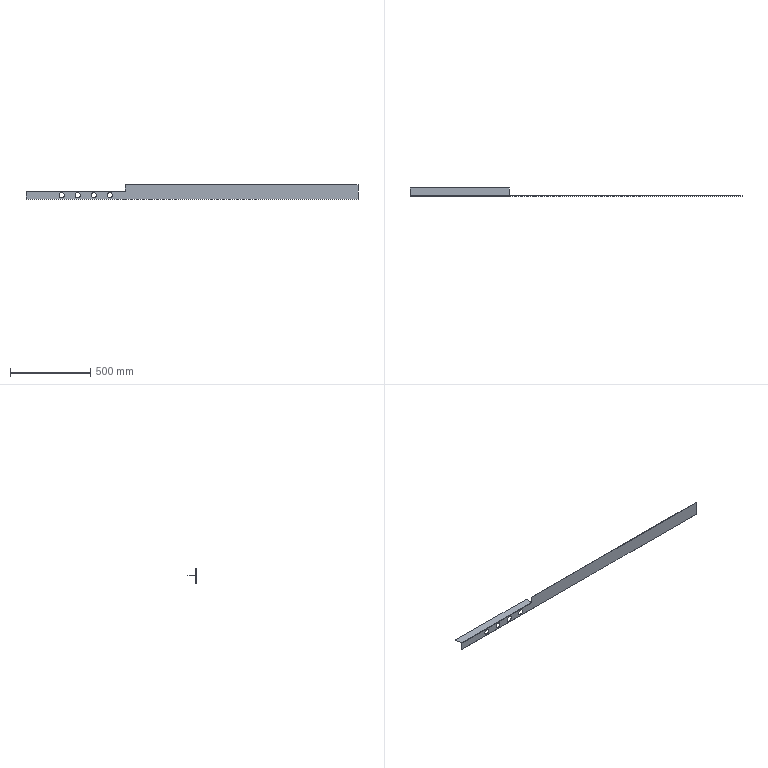Part | STEP file | Baffle 3 | 1 solid | 28 faces | box 2070 x 50 x 90 mm | volume 281521 mm3 | plane 18 | cylinder 10 | commonest cylinder face diameters 33 x8 2 x1 5 x1
STEP:
#1=CARTESIAN_POINT('',(522.5,-1.5,-41.5));
#2=VERTEX_POINT('',#1);
#3=CARTESIAN_POINT('',(522.5,-1.5,-8.5));
#4=VERTEX_POINT('',#3);
#5=CARTESIAN_POINT('',(522.5,-1.5,-25.));
#6=DIRECTION('',(0.,1.,0.));
#7=DIRECTION('',(0.,0.,1.));
#8=AXIS2_PLACEMENT_3D('',#5,#6,#7);
#9=CIRCLE('',#8,16.5);
#10=EDGE_CURVE('',#2,#4,#9,.T.);
#11=ORIENTED_EDGE('',*,*,#10,.F.);
#12=CARTESIAN_POINT('',(522.5,0.,-41.5));
#13=VERTEX_POINT('',#12);
#14=CARTESIAN_POINT('',(522.5,-10.,-41.5));
#15=DIRECTION('',(0.,1.,0.));
#16=VECTOR('',#15,1000.);
#17=LINE('',#14,#16);
#18=EDGE_CURVE('',#2,#13,#17,.T.);
#19=ORIENTED_EDGE('',*,*,#18,.T.);
#20=CARTESIAN_POINT('',(522.5,0.,-8.5));
#21=VERTEX_POINT('',#20);
#22=CARTESIAN_POINT('',(522.5,0.,-25.));
#23=DIRECTION('',(0.,1.,0.));
#24=DIRECTION('',(0.,0.,1.));
#25=AXIS2_PLACEMENT_3D('',#22,#23,#24);
#26=CIRCLE('',#25,16.5);
#27=EDGE_CURVE('',#13,#21,#26,.T.);
#28=ORIENTED_EDGE('',*,*,#27,.T.);
#29=CARTESIAN_POINT('',(522.5,-10.,-8.5));
#30=DIRECTION('',(0.,1.,0.));
#31=VECTOR('',#30,1000.);
#32=LINE('',#29,#31);
#33=EDGE_CURVE('',#4,#21,#32,.T.);
#34=ORIENTED_EDGE('',*,*,#33,.F.);
#35=EDGE_LOOP('',(#11,#19,#28,#34));
#36=FACE_OUTER_BOUND('',#35,.T.);
#37=CARTESIAN_POINT('',(522.5,-10.,-25.));
#38=DIRECTION('',(0.,1.,0.));
#39=DIRECTION('',(0.,0.,1.));
#40=AXIS2_PLACEMENT_3D('',#37,#38,#39);
#41=CYLINDRICAL_SURFACE('',#40,16.5);
#42=ADVANCED_FACE('',(#36),#41,.F.);
#43=CARTESIAN_POINT('',(422.5,-1.5,-41.5));
#44=VERTEX_POINT('',#43);
#45=CARTESIAN_POINT('',(422.5,-1.5,-8.5));
#46=VERTEX_POINT('',#45);
#47=CARTESIAN_POINT('',(422.5,-1.5,-25.));
#48=DIRECTION('',(0.,1.,0.));
#49=DIRECTION('',(0.,0.,1.));
#50=AXIS2_PLACEMENT_3D('',#47,#48,#49);
#51=CIRCLE('',#50,16.5);
#52=EDGE_CURVE('',#44,#46,#51,.T.);
#53=ORIENTED_EDGE('',*,*,#52,.F.);
#54=CARTESIAN_POINT('',(422.5,0.,-41.5));
#55=VERTEX_POINT('',#54);
#56=CARTESIAN_POINT('',(422.5,-10.,-41.5));
#57=DIRECTION('',(0.,1.,0.));
#58=VECTOR('',#57,1000.);
#59=LINE('',#56,#58);
#60=EDGE_CURVE('',#44,#55,#59,.T.);
#61=ORIENTED_EDGE('',*,*,#60,.T.);
#62=CARTESIAN_POINT('',(422.5,0.,-8.5));
#63=VERTEX_POINT('',#62);
#64=CARTESIAN_POINT('',(422.5,0.,-25.));
#65=DIRECTION('',(0.,1.,0.));
#66=DIRECTION('',(0.,0.,1.));
#67=AXIS2_PLACEMENT_3D('',#64,#65,#66);
#68=CIRCLE('',#67,16.5);
#69=EDGE_CURVE('',#55,#63,#68,.T.);
#70=ORIENTED_EDGE('',*,*,#69,.T.);
#71=CARTESIAN_POINT('',(422.5,-10.,-8.5));
#72=DIRECTION('',(0.,1.,0.));
#73=VECTOR('',#72,1000.);
#74=LINE('',#71,#73);
#75=EDGE_CURVE('',#46,#63,#74,.T.);
#76=ORIENTED_EDGE('',*,*,#75,.F.);
#77=EDGE_LOOP('',(#53,#61,#70,#76));
#78=FACE_OUTER_BOUND('',#77,.T.);
#79=CARTESIAN_POINT('',(422.5,-10.,-25.));
#80=DIRECTION('',(0.,1.,0.));
#81=DIRECTION('',(0.,0.,1.));
#82=AXIS2_PLACEMENT_3D('',#79,#80,#81);
#83=CYLINDRICAL_SURFACE('',#82,16.5);
#84=ADVANCED_FACE('',(#78),#83,.F.);
#85=CARTESIAN_POINT('',(322.5,-1.5,-41.5));
#86=VERTEX_POINT('',#85);
#87=CARTESIAN_POINT('',(322.5,-1.5,-8.5));
#88=VERTEX_POINT('',#87);
#89=CARTESIAN_POINT('',(322.5,-1.5,-25.));
#90=DIRECTION('',(0.,1.,0.));
#91=DIRECTION('',(0.,0.,1.));
#92=AXIS2_PLACEMENT_3D('',#89,#90,#91);
#93=CIRCLE('',#92,16.5);
#94=EDGE_CURVE('',#86,#88,#93,.T.);
#95=ORIENTED_EDGE('',*,*,#94,.F.);
#96=CARTESIAN_POINT('',(322.5,0.,-41.5));
#97=VERTEX_POINT('',#96);
#98=CARTESIAN_POINT('',(322.5,-10.,-41.5));
#99=DIRECTION('',(0.,1.,0.));
#100=VECTOR('',#99,1000.);
#101=LINE('',#98,#100);
#102=EDGE_CURVE('',#86,#97,#101,.T.);
#103=ORIENTED_EDGE('',*,*,#102,.T.);
#104=CARTESIAN_POINT('',(322.5,0.,-8.5));
#105=VERTEX_POINT('',#104);
#106=CARTESIAN_POINT('',(322.5,0.,-25.));
#107=DIRECTION('',(0.,1.,0.));
#108=DIRECTION('',(0.,0.,1.));
#109=AXIS2_PLACEMENT_3D('',#106,#107,#108);
#110=CIRCLE('',#109,16.5);
#111=EDGE_CURVE('',#97,#105,#110,.T.);
#112=ORIENTED_EDGE('',*,*,#111,.T.);
#113=CARTESIAN_POINT('',(322.5,-10.,-8.5));
#114=DIRECTION('',(0.,1.,0.));
#115=VECTOR('',#114,1000.);
#116=LINE('',#113,#115);
#117=EDGE_CURVE('',#88,#105,#116,.T.);
#118=ORIENTED_EDGE('',*,*,#117,.F.);
#119=EDGE_LOOP('',(#95,#103,#112,#118));
#120=FACE_OUTER_BOUND('',#119,.T.);
#121=CARTESIAN_POINT('',(322.5,-10.,-25.));
#122=DIRECTION('',(0.,1.,0.));
#123=DIRECTION('',(0.,0.,1.));
#124=AXIS2_PLACEMENT_3D('',#121,#122,#123);
#125=CYLINDRICAL_SURFACE('',#124,16.5);
#126=ADVANCED_FACE('',(#120),#125,.F.);
#127=CARTESIAN_POINT('',(222.5,-1.5,-41.5));
#128=VERTEX_POINT('',#127);
#129=CARTESIAN_POINT('',(222.5,-1.5,-8.5));
#130=VERTEX_POINT('',#129);
#131=CARTESIAN_POINT('',(222.5,-1.5,-25.));
#132=DIRECTION('',(0.,1.,0.));
#133=DIRECTION('',(0.,0.,1.));
#134=AXIS2_PLACEMENT_3D('',#131,#132,#133);
#135=CIRCLE('',#134,16.5);
#136=EDGE_CURVE('',#128,#130,#135,.T.);
#137=ORIENTED_EDGE('',*,*,#136,.F.);
#138=CARTESIAN_POINT('',(222.5,0.,-41.5));
#139=VERTEX_POINT('',#138);
#140=CARTESIAN_POINT('',(222.5,-10.,-41.5));
#141=DIRECTION('',(0.,1.,0.));
#142=VECTOR('',#141,1000.);
#143=LINE('',#140,#142);
#144=EDGE_CURVE('',#128,#139,#143,.T.);
#145=ORIENTED_EDGE('',*,*,#144,.T.);
#146=CARTESIAN_POINT('',(222.5,0.,-8.5));
#147=VERTEX_POINT('',#146);
#148=CARTESIAN_POINT('',(222.5,0.,-25.));
#149=DIRECTION('',(0.,1.,0.));
#150=DIRECTION('',(0.,0.,1.));
#151=AXIS2_PLACEMENT_3D('',#148,#149,#150);
#152=CIRCLE('',#151,16.5);
#153=EDGE_CURVE('',#139,#147,#152,.T.);
#154=ORIENTED_EDGE('',*,*,#153,.T.);
#155=CARTESIAN_POINT('',(222.5,-10.,-8.5));
#156=DIRECTION('',(0.,1.,0.));
#157=VECTOR('',#156,1000.);
#158=LINE('',#155,#157);
#159=EDGE_CURVE('',#130,#147,#158,.T.);
#160=ORIENTED_EDGE('',*,*,#159,.F.);
#161=EDGE_LOOP('',(#137,#145,#154,#160));
#162=FACE_OUTER_BOUND('',#161,.T.);
#163=CARTESIAN_POINT('',(222.5,-10.,-25.));
#164=DIRECTION('',(0.,1.,0.));
#165=DIRECTION('',(0.,0.,1.));
#166=AXIS2_PLACEMENT_3D('',#163,#164,#165);
#167=CYLINDRICAL_SURFACE('',#166,16.5);
#168=ADVANCED_FACE('',(#162),#167,.F.);
#169=CARTESIAN_POINT('',(522.5,-1.5,-25.));
#170=DIRECTION('',(0.,1.,0.));
#171=DIRECTION('',(0.,0.,1.));
#172=AXIS2_PLACEMENT_3D('',#169,#170,#171);
#173=CIRCLE('',#172,16.5);
#174=EDGE_CURVE('',#4,#2,#173,.T.);
#175=ORIENTED_EDGE('',*,*,#174,.T.);
#176=ORIENTED_EDGE('',*,*,#10,.T.);
#177=EDGE_LOOP('',(#175,#176));
#178=FACE_BOUND('',#177,.T.);
#179=CARTESIAN_POINT('',(422.5,-1.5,-25.));
#180=DIRECTION('',(0.,1.,0.));
#181=DIRECTION('',(0.,0.,1.));
#182=AXIS2_PLACEMENT_3D('',#179,#180,#181);
#183=CIRCLE('',#182,16.5);
#184=EDGE_CURVE('',#46,#44,#183,.T.);
#185=ORIENTED_EDGE('',*,*,#184,.T.);
#186=ORIENTED_EDGE('',*,*,#52,.T.);
#187=EDGE_LOOP('',(#185,#186));
#188=FACE_BOUND('',#187,.T.);
#189=CARTESIAN_POINT('',(322.5,-1.5,-25.));
#190=DIRECTION('',(0.,1.,0.));
#191=DIRECTION('',(0.,0.,1.));
#192=AXIS2_PLACEMENT_3D('',#189,#190,#191);
#193=CIRCLE('',#192,16.5);
#194=EDGE_CURVE('',#88,#86,#193,.T.);
#195=ORIENTED_EDGE('',*,*,#194,.T.);
#196=ORIENTED_EDGE('',*,*,#94,.T.);
#197=EDGE_LOOP('',(#195,#196));
#198=FACE_BOUND('',#197,.T.);
#199=CARTESIAN_POINT('',(222.5,-1.5,-25.));
#200=DIRECTION('',(0.,1.,0.));
#201=DIRECTION('',(0.,0.,1.));
#202=AXIS2_PLACEMENT_3D('',#199,#200,#201);
#203=CIRCLE('',#202,16.5);
#204=EDGE_CURVE('',#130,#128,#203,.T.);
#205=ORIENTED_EDGE('',*,*,#204,.T.);
#206=ORIENTED_EDGE('',*,*,#136,.T.);
#207=EDGE_LOOP('',(#205,#206));
#208=FACE_BOUND('',#207,.T.);
#209=CARTESIAN_POINT('',(620.75,-1.5,0.));
#210=VERTEX_POINT('',#209);
#211=CARTESIAN_POINT('',(620.,-1.5,0.));
#212=VERTEX_POINT('',#211);
#213=CARTESIAN_POINT('',(0.,-1.5,0.));
#214=DIRECTION('',(-1.,0.,0.));
#215=VECTOR('',#214,1000.);
#216=LINE('',#213,#215);
#217=EDGE_CURVE('',#210,#212,#216,.T.);
#218=ORIENTED_EDGE('',*,*,#217,.F.);
#219=CARTESIAN_POINT('',(620.75,-1.5,-3.25));
#220=VERTEX_POINT('',#219);
#221=CARTESIAN_POINT('',(620.75,-1.5,0.));
#222=DIRECTION('',(0.,0.,1.));
#223=VECTOR('',#222,1000.);
#224=LINE('',#221,#223);
#225=EDGE_CURVE('',#220,#210,#224,.T.);
#226=ORIENTED_EDGE('',*,*,#225,.F.);
#227=CARTESIAN_POINT('',(620.,-1.5,-3.25));
#228=VERTEX_POINT('',#227);
#229=CARTESIAN_POINT('',(0.,-1.5,-3.25));
#230=DIRECTION('',(1.,0.,0.));
#231=VECTOR('',#230,1000.);
#232=LINE('',#229,#231);
#233=EDGE_CURVE('',#228,#220,#232,.T.);
#234=ORIENTED_EDGE('',*,*,#233,.F.);
#235=CARTESIAN_POINT('',(620.,-1.5,-2.5));
#236=VERTEX_POINT('',#235);
#237=CARTESIAN_POINT('',(620.,-1.5,0.));
#238=DIRECTION('',(0.,0.,-1.));
#239=VECTOR('',#238,1000.);
#240=LINE('',#237,#239);
#241=EDGE_CURVE('',#236,#228,#240,.T.);
#242=ORIENTED_EDGE('',*,*,#241,.F.);
#243=CARTESIAN_POINT('',(0.,-1.5,-2.5));
#244=VERTEX_POINT('',#243);
#245=CARTESIAN_POINT('',(620.,-1.5,-2.5));
#246=DIRECTION('',(-1.,0.,0.));
#247=VECTOR('',#246,1000.);
#248=LINE('',#245,#247);
#249=EDGE_CURVE('',#236,#244,#248,.T.);
#250=ORIENTED_EDGE('',*,*,#249,.T.);
#251=CARTESIAN_POINT('',(0.,-1.5,-50.));
#252=VERTEX_POINT('',#251);
#253=CARTESIAN_POINT('',(0.,-1.5,-50.));
#254=DIRECTION('',(0.,0.,1.));
#255=VECTOR('',#254,1000.);
#256=LINE('',#253,#255);
#257=EDGE_CURVE('',#252,#244,#256,.T.);
#258=ORIENTED_EDGE('',*,*,#257,.F.);
#259=CARTESIAN_POINT('',(2070.,-1.5,-50.));
#260=VERTEX_POINT('',#259);
#261=CARTESIAN_POINT('',(2070.,-1.5,-50.));
#262=DIRECTION('',(-1.,0.,0.));
#263=VECTOR('',#262,1000.);
#264=LINE('',#261,#263);
#265=EDGE_CURVE('',#260,#252,#264,.T.);
#266=ORIENTED_EDGE('',*,*,#265,.F.);
#267=CARTESIAN_POINT('',(2070.,-1.5,40.));
#268=VERTEX_POINT('',#267);
#269=CARTESIAN_POINT('',(2070.,-1.5,40.));
#270=DIRECTION('',(0.,0.,-1.));
#271=VECTOR('',#270,1000.);
#272=LINE('',#269,#271);
#273=EDGE_CURVE('',#268,#260,#272,.T.);
#274=ORIENTED_EDGE('',*,*,#273,.F.);
#275=CARTESIAN_POINT('',(620.,-1.5,40.));
#276=VERTEX_POINT('',#275);
#277=CARTESIAN_POINT('',(620.,-1.5,40.));
#278=DIRECTION('',(1.,0.,0.));
#279=VECTOR('',#278,1000.);
#280=LINE('',#277,#279);
#281=EDGE_CURVE('',#276,#268,#280,.T.);
#282=ORIENTED_EDGE('',*,*,#281,.F.);
#283=CARTESIAN_POINT('',(620.,-1.5,0.));
#284=DIRECTION('',(0.,0.,1.));
#285=VECTOR('',#284,1000.);
#286=LINE('',#283,#285);
#287=EDGE_CURVE('',#212,#276,#286,.T.);
#288=ORIENTED_EDGE('',*,*,#287,.F.);
#289=EDGE_LOOP('',(#218,#226,#234,#242,#250,#258,#266,#274,#282,#288));
#290=FACE_OUTER_BOUND('',#289,.T.);
#291=CARTESIAN_POINT('',(0.,-1.5,0.));
#292=DIRECTION('',(0.,1.,0.));
#293=DIRECTION('',(0.,0.,1.));
#294=AXIS2_PLACEMENT_3D('',#291,#292,#293);
#295=PLANE('',#294);
#296=ADVANCED_FACE('',(#178,#188,#198,#208,#290),#295,.F.);
#297=CARTESIAN_POINT('',(522.5,0.,-25.));
#298=DIRECTION('',(0.,1.,0.));
#299=DIRECTION('',(0.,0.,1.));
#300=AXIS2_PLACEMENT_3D('',#297,#298,#299);
#301=CIRCLE('',#300,16.5);
#302=EDGE_CURVE('',#21,#13,#301,.T.);
#303=ORIENTED_EDGE('',*,*,#302,.F.);
#304=ORIENTED_EDGE('',*,*,#27,.F.);
#305=EDGE_LOOP('',(#303,#304));
#306=FACE_BOUND('',#305,.T.);
#307=CARTESIAN_POINT('',(422.5,0.,-25.));
#308=DIRECTION('',(0.,1.,0.));
#309=DIRECTION('',(0.,0.,1.));
#310=AXIS2_PLACEMENT_3D('',#307,#308,#309);
#311=CIRCLE('',#310,16.5);
#312=EDGE_CURVE('',#63,#55,#311,.T.);
#313=ORIENTED_EDGE('',*,*,#312,.F.);
#314=ORIENTED_EDGE('',*,*,#69,.F.);
#315=EDGE_LOOP('',(#313,#314));
#316=FACE_BOUND('',#315,.T.);
#317=CARTESIAN_POINT('',(322.5,0.,-25.));
#318=DIRECTION('',(0.,1.,0.));
#319=DIRECTION('',(0.,0.,1.));
#320=AXIS2_PLACEMENT_3D('',#317,#318,#319);
#321=CIRCLE('',#320,16.5);
#322=EDGE_CURVE('',#105,#97,#321,.T.);
#323=ORIENTED_EDGE('',*,*,#322,.F.);
#324=ORIENTED_EDGE('',*,*,#111,.F.);
#325=EDGE_LOOP('',(#323,#324));
#326=FACE_BOUND('',#325,.T.);
#327=CARTESIAN_POINT('',(222.5,0.,-25.));
#328=DIRECTION('',(0.,1.,0.));
#329=DIRECTION('',(0.,0.,1.));
#330=AXIS2_PLACEMENT_3D('',#327,#328,#329);
#331=CIRCLE('',#330,16.5);
#332=EDGE_CURVE('',#147,#139,#331,.T.);
#333=ORIENTED_EDGE('',*,*,#332,.F.);
#334=ORIENTED_EDGE('',*,*,#153,.F.);
#335=EDGE_LOOP('',(#333,#334));
#336=FACE_BOUND('',#335,.T.);
#337=CARTESIAN_POINT('',(620.75,0.,0.));
#338=VERTEX_POINT('',#337);
#339=CARTESIAN_POINT('',(620.75,0.,-3.25));
#340=VERTEX_POINT('',#339);
#341=CARTESIAN_POINT('',(620.75,0.,0.));
#342=DIRECTION('',(0.,0.,-1.));
#343=VECTOR('',#342,1000.);
#344=LINE('',#341,#343);
#345=EDGE_CURVE('',#338,#340,#344,.T.);
#346=ORIENTED_EDGE('',*,*,#345,.F.);
#347=CARTESIAN_POINT('',(620.,0.,0.));
#348=VERTEX_POINT('',#347);
#349=CARTESIAN_POINT('',(620.,0.,0.));
#350=DIRECTION('',(1.,0.,0.));
#351=VECTOR('',#350,1000.);
#352=LINE('',#349,#351);
#353=EDGE_CURVE('',#348,#338,#352,.T.);
#354=ORIENTED_EDGE('',*,*,#353,.F.);
#355=CARTESIAN_POINT('',(620.,0.,40.));
#356=VERTEX_POINT('',#355);
#357=CARTESIAN_POINT('',(620.,0.,0.));
#358=DIRECTION('',(0.,0.,1.));
#359=VECTOR('',#358,1000.);
#360=LINE('',#357,#359);
#361=EDGE_CURVE('',#348,#356,#360,.T.);
#362=ORIENTED_EDGE('',*,*,#361,.T.);
#363=CARTESIAN_POINT('',(2070.,0.,40.));
#364=VERTEX_POINT('',#363);
#365=CARTESIAN_POINT('',(620.,0.,40.));
#366=DIRECTION('',(1.,0.,0.));
#367=VECTOR('',#366,1000.);
#368=LINE('',#365,#367);
#369=EDGE_CURVE('',#356,#364,#368,.T.);
#370=ORIENTED_EDGE('',*,*,#369,.T.);
#371=CARTESIAN_POINT('',(2070.,0.,-50.));
#372=VERTEX_POINT('',#371);
#373=CARTESIAN_POINT('',(2070.,0.,40.));
#374=DIRECTION('',(0.,0.,-1.));
#375=VECTOR('',#374,1000.);
#376=LINE('',#373,#375);
#377=EDGE_CURVE('',#364,#372,#376,.T.);
#378=ORIENTED_EDGE('',*,*,#377,.T.);
#379=CARTESIAN_POINT('',(0.,0.,-50.));
#380=VERTEX_POINT('',#379);
#381=CARTESIAN_POINT('',(2070.,0.,-50.));
#382=DIRECTION('',(-1.,0.,0.));
#383=VECTOR('',#382,1000.);
#384=LINE('',#381,#383);
#385=EDGE_CURVE('',#372,#380,#384,.T.);
#386=ORIENTED_EDGE('',*,*,#385,.T.);
#387=CARTESIAN_POINT('',(0.,0.,-2.5));
#388=VERTEX_POINT('',#387);
#389=CARTESIAN_POINT('',(0.,0.,-50.));
#390=DIRECTION('',(0.,0.,1.));
#391=VECTOR('',#390,1000.);
#392=LINE('',#389,#391);
#393=EDGE_CURVE('',#380,#388,#392,.T.);
#394=ORIENTED_EDGE('',*,*,#393,.T.);
#395=CARTESIAN_POINT('',(620.,0.,-2.5));
#396=VERTEX_POINT('',#395);
#397=CARTESIAN_POINT('',(620.,0.,-2.5));
#398=DIRECTION('',(-1.,0.,0.));
#399=VECTOR('',#398,1000.);
#400=LINE('',#397,#399);
#401=EDGE_CURVE('',#396,#388,#400,.T.);
#402=ORIENTED_EDGE('',*,*,#401,.F.);
#403=CARTESIAN_POINT('',(620.,0.,-3.25));
#404=VERTEX_POINT('',#403);
#405=CARTESIAN_POINT('',(620.,0.,-3.25));
#406=DIRECTION('',(0.,0.,1.));
#407=VECTOR('',#406,1000.);
#408=LINE('',#405,#407);
#409=EDGE_CURVE('',#404,#396,#408,.T.);
#410=ORIENTED_EDGE('',*,*,#409,.F.);
#411=CARTESIAN_POINT('',(620.75,0.,-3.25));
#412=DIRECTION('',(-1.,0.,0.));
#413=VECTOR('',#412,1000.);
#414=LINE('',#411,#413);
#415=EDGE_CURVE('',#340,#404,#414,.T.);
#416=ORIENTED_EDGE('',*,*,#415,.F.);
#417=EDGE_LOOP('',(#346,#354,#362,#370,#378,#386,#394,#402,#410,#416));
#418=FACE_OUTER_BOUND('',#417,.T.);
#419=CARTESIAN_POINT('',(0.,0.,0.));
#420=DIRECTION('',(0.,1.,0.));
#421=DIRECTION('',(0.,0.,1.));
#422=AXIS2_PLACEMENT_3D('',#419,#420,#421);
#423=PLANE('',#422);
#424=ADVANCED_FACE('',(#306,#316,#326,#336,#418),#423,.T.);
#425=CARTESIAN_POINT('',(0.,0.,-2.5));
#426=DIRECTION('',(0.,-1.,0.));
#427=VECTOR('',#426,1000.);
#428=LINE('',#425,#427);
#429=EDGE_CURVE('',#388,#244,#428,.T.);
#430=ORIENTED_EDGE('',*,*,#429,.F.);
#431=ORIENTED_EDGE('',*,*,#393,.F.);
#432=CARTESIAN_POINT('',(0.,-1.5,-50.));
#433=DIRECTION('',(0.,1.,0.));
#434=VECTOR('',#433,1000.);
#435=LINE('',#432,#434);
#436=EDGE_CURVE('',#252,#380,#435,.T.);
#437=ORIENTED_EDGE('',*,*,#436,.F.);
#438=ORIENTED_EDGE('',*,*,#257,.T.);
#439=EDGE_LOOP('',(#430,#431,#437,#438));
#440=FACE_OUTER_BOUND('',#439,.T.);
#441=CARTESIAN_POINT('',(0.,-1.5,-50.));
#442=DIRECTION('',(-1.,0.,0.));
#443=DIRECTION('',(0.,0.,1.));
#444=AXIS2_PLACEMENT_3D('',#441,#442,#443);
#445=PLANE('',#444);
#446=ADVANCED_FACE('',(#440),#445,.T.);
#447=ORIENTED_EDGE('',*,*,#385,.F.);
#448=CARTESIAN_POINT('',(2070.,-1.5,-50.));
#449=DIRECTION('',(0.,1.,0.));
#450=VECTOR('',#449,1000.);
#451=LINE('',#448,#450);
#452=EDGE_CURVE('',#260,#372,#451,.T.);
#453=ORIENTED_EDGE('',*,*,#452,.F.);
#454=ORIENTED_EDGE('',*,*,#265,.T.);
#455=ORIENTED_EDGE('',*,*,#436,.T.);
#456=EDGE_LOOP('',(#447,#453,#454,#455));
#457=FACE_OUTER_BOUND('',#456,.T.);
#458=CARTESIAN_POINT('',(2070.,-1.5,-50.));
#459=DIRECTION('',(0.,0.,-1.));
#460=DIRECTION('',(-1.,0.,0.));
#461=AXIS2_PLACEMENT_3D('',#458,#459,#460);
#462=PLANE('',#461);
#463=ADVANCED_FACE('',(#457),#462,.T.);
#464=ORIENTED_EDGE('',*,*,#377,.F.);
#465=CARTESIAN_POINT('',(2070.,-1.5,40.));
#466=DIRECTION('',(0.,1.,0.));
#467=VECTOR('',#466,1000.);
#468=LINE('',#465,#467);
#469=EDGE_CURVE('',#268,#364,#468,.T.);
#470=ORIENTED_EDGE('',*,*,#469,.F.);
#471=ORIENTED_EDGE('',*,*,#273,.T.);
#472=ORIENTED_EDGE('',*,*,#452,.T.);
#473=EDGE_LOOP('',(#464,#470,#471,#472));
#474=FACE_OUTER_BOUND('',#473,.T.);
#475=CARTESIAN_POINT('',(2070.,-1.5,40.));
#476=DIRECTION('',(1.,0.,0.));
#477=DIRECTION('',(0.,0.,-1.));
#478=AXIS2_PLACEMENT_3D('',#475,#476,#477);
#479=PLANE('',#478);
#480=ADVANCED_FACE('',(#474),#479,.T.);
#481=ORIENTED_EDGE('',*,*,#369,.F.);
#482=CARTESIAN_POINT('',(620.,-1.5,40.));
#483=DIRECTION('',(0.,1.,0.));
#484=VECTOR('',#483,1000.);
#485=LINE('',#482,#484);
#486=EDGE_CURVE('',#276,#356,#485,.T.);
#487=ORIENTED_EDGE('',*,*,#486,.F.);
#488=ORIENTED_EDGE('',*,*,#281,.T.);
#489=ORIENTED_EDGE('',*,*,#469,.T.);
#490=EDGE_LOOP('',(#481,#487,#488,#489));
#491=FACE_OUTER_BOUND('',#490,.T.);
#492=CARTESIAN_POINT('',(620.,-1.5,40.));
#493=DIRECTION('',(0.,0.,1.));
#494=DIRECTION('',(1.,0.,0.));
#495=AXIS2_PLACEMENT_3D('',#492,#493,#494);
#496=PLANE('',#495);
#497=ADVANCED_FACE('',(#491),#496,.T.);
#498=ORIENTED_EDGE('',*,*,#361,.F.);
#499=CARTESIAN_POINT('',(620.,-1.5,0.));
#500=DIRECTION('',(0.,1.,0.));
#501=VECTOR('',#500,1000.);
#502=LINE('',#499,#501);
#503=EDGE_CURVE('',#212,#348,#502,.T.);
#504=ORIENTED_EDGE('',*,*,#503,.F.);
#505=ORIENTED_EDGE('',*,*,#287,.T.);
#506=ORIENTED_EDGE('',*,*,#486,.T.);
#507=EDGE_LOOP('',(#498,#504,#505,#506));
#508=FACE_OUTER_BOUND('',#507,.T.);
#509=CARTESIAN_POINT('',(620.,-1.5,0.));
#510=DIRECTION('',(-1.,0.,0.));
#511=DIRECTION('',(0.,0.,1.));
#512=AXIS2_PLACEMENT_3D('',#509,#510,#511);
#513=PLANE('',#512);
#514=ADVANCED_FACE('',(#508),#513,.T.);
#515=CARTESIAN_POINT('',(620.75,0.,0.));
#516=DIRECTION('',(0.,-1.,0.));
#517=VECTOR('',#516,1000.);
#518=LINE('',#515,#517);
#519=EDGE_CURVE('',#338,#210,#518,.T.);
#520=ORIENTED_EDGE('',*,*,#519,.T.);
#521=ORIENTED_EDGE('',*,*,#217,.T.);
#522=ORIENTED_EDGE('',*,*,#503,.T.);
#523=ORIENTED_EDGE('',*,*,#353,.T.);
#524=EDGE_LOOP('',(#520,#521,#522,#523));
#525=FACE_OUTER_BOUND('',#524,.T.);
#526=CARTESIAN_POINT('',(620.,0.,0.));
#527=DIRECTION('',(0.,0.,-1.));
#528=DIRECTION('',(0.,1.,0.));
#529=AXIS2_PLACEMENT_3D('',#526,#527,#528);
#530=PLANE('',#529);
#531=ADVANCED_FACE('',(#525),#530,.T.);
#532=CARTESIAN_POINT('',(620.75,0.,-3.25));
#533=DIRECTION('',(0.,-1.,0.));
#534=VECTOR('',#533,1000.);
#535=LINE('',#532,#534);
#536=EDGE_CURVE('',#340,#220,#535,.T.);
#537=ORIENTED_EDGE('',*,*,#536,.T.);
#538=ORIENTED_EDGE('',*,*,#225,.T.);
#539=ORIENTED_EDGE('',*,*,#519,.F.);
#540=ORIENTED_EDGE('',*,*,#345,.T.);
#541=EDGE_LOOP('',(#537,#538,#539,#540));
#542=FACE_OUTER_BOUND('',#541,.T.);
#543=CARTESIAN_POINT('',(620.75,0.,0.));
#544=DIRECTION('',(-1.,0.,0.));
#545=DIRECTION('',(0.,0.,1.));
#546=AXIS2_PLACEMENT_3D('',#543,#544,#545);
#547=PLANE('',#546);
#548=ADVANCED_FACE('',(#542),#547,.T.);
#549=CARTESIAN_POINT('',(620.,0.,-3.25));
#550=DIRECTION('',(0.,-1.,0.));
#551=VECTOR('',#550,1000.);
#552=LINE('',#549,#551);
#553=EDGE_CURVE('',#404,#228,#552,.T.);
#554=ORIENTED_EDGE('',*,*,#553,.T.);
#555=ORIENTED_EDGE('',*,*,#233,.T.);
#556=ORIENTED_EDGE('',*,*,#536,.F.);
#557=ORIENTED_EDGE('',*,*,#415,.T.);
#558=EDGE_LOOP('',(#554,#555,#556,#557));
#559=FACE_OUTER_BOUND('',#558,.T.);
#560=CARTESIAN_POINT('',(620.75,0.,-3.25));
#561=DIRECTION('',(0.,0.,1.));
#562=DIRECTION('',(0.,-1.,0.));
#563=AXIS2_PLACEMENT_3D('',#560,#561,#562);
#564=PLANE('',#563);
#565=ADVANCED_FACE('',(#559),#564,.T.);
#566=CARTESIAN_POINT('',(620.,0.,-2.5));
#567=DIRECTION('',(0.,-1.,0.));
#568=VECTOR('',#567,1000.);
#569=LINE('',#566,#568);
#570=EDGE_CURVE('',#396,#236,#569,.T.);
#571=ORIENTED_EDGE('',*,*,#570,.T.);
#572=ORIENTED_EDGE('',*,*,#241,.T.);
#573=ORIENTED_EDGE('',*,*,#553,.F.);
#574=ORIENTED_EDGE('',*,*,#409,.T.);
#575=EDGE_LOOP('',(#571,#572,#573,#574));
#576=FACE_OUTER_BOUND('',#575,.T.);
#577=CARTESIAN_POINT('',(620.,0.,-3.25));
#578=DIRECTION('',(1.,0.,0.));
#579=DIRECTION('',(0.,0.,-1.));
#580=AXIS2_PLACEMENT_3D('',#577,#578,#579);
#581=PLANE('',#580);
#582=ADVANCED_FACE('',(#576),#581,.T.);
#583=CARTESIAN_POINT('',(0.,1.,-1.5));
#584=VERTEX_POINT('',#583);
#585=CARTESIAN_POINT('',(0.,1.,0.));
#586=VERTEX_POINT('',#585);
#587=CARTESIAN_POINT('',(0.,1.,0.));
#588=DIRECTION('',(0.,0.,1.));
#589=VECTOR('',#588,1000.);
#590=LINE('',#587,#589);
#591=EDGE_CURVE('',#584,#586,#590,.T.);
#592=ORIENTED_EDGE('',*,*,#591,.F.);
#593=CARTESIAN_POINT('',(0.,1.,-2.5));
#594=DIRECTION('',(-1.,0.,0.));
#595=DIRECTION('',(0.,0.,-1.));
#596=AXIS2_PLACEMENT_3D('',#593,#594,#595);
#597=CIRCLE('',#596,1.);
#598=EDGE_CURVE('',#388,#584,#597,.T.);
#599=ORIENTED_EDGE('',*,*,#598,.F.);
#600=ORIENTED_EDGE('',*,*,#429,.T.);
#601=CARTESIAN_POINT('',(0.,1.,-2.5));
#602=DIRECTION('',(-1.,0.,0.));
#603=DIRECTION('',(0.,0.,-1.));
#604=AXIS2_PLACEMENT_3D('',#601,#602,#603);
#605=CIRCLE('',#604,2.5);
#606=EDGE_CURVE('',#244,#586,#605,.T.);
#607=ORIENTED_EDGE('',*,*,#606,.T.);
#608=EDGE_LOOP('',(#592,#599,#600,#607));
#609=FACE_OUTER_BOUND('',#608,.T.);
#610=CARTESIAN_POINT('',(0.,1.,-2.5));
#611=DIRECTION('',(-1.,0.,0.));
#612=DIRECTION('',(0.,0.,1.));
#613=AXIS2_PLACEMENT_3D('',#610,#611,#612);
#614=PLANE('',#613);
#615=ADVANCED_FACE('',(#609),#614,.T.);
#616=CARTESIAN_POINT('',(620.,1.,-1.5));
#617=VERTEX_POINT('',#616);
#618=CARTESIAN_POINT('',(620.,1.,-2.5));
#619=DIRECTION('',(1.,0.,0.));
#620=DIRECTION('',(0.,0.,-1.));
#621=AXIS2_PLACEMENT_3D('',#618,#619,#620);
#622=CIRCLE('',#621,1.);
#623=EDGE_CURVE('',#617,#396,#622,.T.);
#624=ORIENTED_EDGE('',*,*,#623,.F.);
#625=CARTESIAN_POINT('',(620.,1.,0.));
#626=VERTEX_POINT('',#625);
#627=CARTESIAN_POINT('',(620.,1.,-1.5));
#628=DIRECTION('',(0.,0.,1.));
#629=VECTOR('',#628,1000.);
#630=LINE('',#627,#629);
#631=EDGE_CURVE('',#617,#626,#630,.T.);
#632=ORIENTED_EDGE('',*,*,#631,.T.);
#633=CARTESIAN_POINT('',(620.,1.,-2.5));
#634=DIRECTION('',(1.,0.,0.));
#635=DIRECTION('',(0.,0.,-1.));
#636=AXIS2_PLACEMENT_3D('',#633,#634,#635);
#637=CIRCLE('',#636,2.5);
#638=EDGE_CURVE('',#626,#236,#637,.T.);
#639=ORIENTED_EDGE('',*,*,#638,.T.);
#640=ORIENTED_EDGE('',*,*,#570,.F.);
#641=EDGE_LOOP('',(#624,#632,#639,#640));
#642=FACE_OUTER_BOUND('',#641,.T.);
#643=CARTESIAN_POINT('',(620.,1.,-2.5));
#644=DIRECTION('',(-1.,0.,0.));
#645=DIRECTION('',(0.,0.,1.));
#646=AXIS2_PLACEMENT_3D('',#643,#644,#645);
#647=PLANE('',#646);
#648=ADVANCED_FACE('',(#642),#647,.F.);
#649=ORIENTED_EDGE('',*,*,#249,.F.);
#650=ORIENTED_EDGE('',*,*,#638,.F.);
#651=CARTESIAN_POINT('',(0.,1.,0.));
#652=DIRECTION('',(-1.,0.,0.));
#653=VECTOR('',#652,1000.);
#654=LINE('',#651,#653);
#655=EDGE_CURVE('',#626,#586,#654,.T.);
#656=ORIENTED_EDGE('',*,*,#655,.T.);
#657=ORIENTED_EDGE('',*,*,#606,.F.);
#658=EDGE_LOOP('',(#649,#650,#656,#657));
#659=FACE_OUTER_BOUND('',#658,.T.);
#660=CARTESIAN_POINT('',(620.,1.,-2.5));
#661=DIRECTION('',(1.,0.,0.));
#662=DIRECTION('',(0.,0.,1.));
#663=AXIS2_PLACEMENT_3D('',#660,#661,#662);
#664=CYLINDRICAL_SURFACE('',#663,2.5);
#665=ADVANCED_FACE('',(#659),#664,.T.);
#666=ORIENTED_EDGE('',*,*,#401,.T.);
#667=ORIENTED_EDGE('',*,*,#598,.T.);
#668=CARTESIAN_POINT('',(0.,1.,-1.5));
#669=DIRECTION('',(1.,0.,0.));
#670=VECTOR('',#669,1000.);
#671=LINE('',#668,#670);
#672=EDGE_CURVE('',#584,#617,#671,.T.);
#673=ORIENTED_EDGE('',*,*,#672,.T.);
#674=ORIENTED_EDGE('',*,*,#623,.T.);
#675=EDGE_LOOP('',(#666,#667,#673,#674));
#676=FACE_OUTER_BOUND('',#675,.T.);
#677=CARTESIAN_POINT('',(620.,1.,-2.5));
#678=DIRECTION('',(1.,0.,0.));
#679=DIRECTION('',(0.,0.,1.));
#680=AXIS2_PLACEMENT_3D('',#677,#678,#679);
#681=CYLINDRICAL_SURFACE('',#680,1.);
#682=ADVANCED_FACE('',(#676),#681,.F.);
#683=ORIENTED_EDGE('',*,*,#591,.T.);
#684=CARTESIAN_POINT('',(0.,48.5,0.));
#685=VERTEX_POINT('',#684);
#686=CARTESIAN_POINT('',(0.,0.,0.));
#687=DIRECTION('',(0.,-1.,0.));
#688=VECTOR('',#687,1000.);
#689=LINE('',#686,#688);
#690=EDGE_CURVE('',#685,#586,#689,.T.);
#691=ORIENTED_EDGE('',*,*,#690,.F.);
#692=CARTESIAN_POINT('',(0.,48.5,-1.5));
#693=VERTEX_POINT('',#692);
#694=CARTESIAN_POINT('',(0.,48.5,0.));
#695=DIRECTION('',(0.,0.,-1.));
#696=VECTOR('',#695,1000.);
#697=LINE('',#694,#696);
#698=EDGE_CURVE('',#685,#693,#697,.T.);
#699=ORIENTED_EDGE('',*,*,#698,.T.);
#700=CARTESIAN_POINT('',(0.,0.,-1.5));
#701=DIRECTION('',(0.,-1.,0.));
#702=VECTOR('',#701,1000.);
#703=LINE('',#700,#702);
#704=EDGE_CURVE('',#693,#584,#703,.T.);
#705=ORIENTED_EDGE('',*,*,#704,.T.);
#706=EDGE_LOOP('',(#683,#691,#699,#705));
#707=FACE_OUTER_BOUND('',#706,.T.);
#708=CARTESIAN_POINT('',(0.,0.,0.));
#709=DIRECTION('',(1.,0.,0.));
#710=DIRECTION('',(0.,0.,-1.));
#711=AXIS2_PLACEMENT_3D('',#708,#709,#710);
#712=PLANE('',#711);
#713=ADVANCED_FACE('',(#707),#712,.F.);
#714=ORIENTED_EDGE('',*,*,#631,.F.);
#715=CARTESIAN_POINT('',(620.,48.5,-1.5));
#716=VERTEX_POINT('',#715);
#717=CARTESIAN_POINT('',(620.,48.5,-1.5));
#718=DIRECTION('',(0.,1.,0.));
#719=VECTOR('',#718,1000.);
#720=LINE('',#717,#719);
#721=EDGE_CURVE('',#617,#716,#720,.T.);
#722=ORIENTED_EDGE('',*,*,#721,.T.);
#723=CARTESIAN_POINT('',(620.,48.5,0.));
#724=VERTEX_POINT('',#723);
#725=CARTESIAN_POINT('',(620.,48.5,0.));
#726=DIRECTION('',(0.,0.,-1.));
#727=VECTOR('',#726,1000.);
#728=LINE('',#725,#727);
#729=EDGE_CURVE('',#724,#716,#728,.T.);
#730=ORIENTED_EDGE('',*,*,#729,.F.);
#731=CARTESIAN_POINT('',(620.,0.,0.));
#732=DIRECTION('',(0.,1.,0.));
#733=VECTOR('',#732,1000.);
#734=LINE('',#731,#733);
#735=EDGE_CURVE('',#626,#724,#734,.T.);
#736=ORIENTED_EDGE('',*,*,#735,.F.);
#737=EDGE_LOOP('',(#714,#722,#730,#736));
#738=FACE_OUTER_BOUND('',#737,.T.);
#739=CARTESIAN_POINT('',(620.,48.5,0.));
#740=DIRECTION('',(-1.,0.,0.));
#741=DIRECTION('',(0.,0.,1.));
#742=AXIS2_PLACEMENT_3D('',#739,#740,#741);
#743=PLANE('',#742);
#744=ADVANCED_FACE('',(#738),#743,.F.);
#745=ORIENTED_EDGE('',*,*,#655,.F.);
#746=ORIENTED_EDGE('',*,*,#735,.T.);
#747=CARTESIAN_POINT('',(0.,48.5,0.));
#748=DIRECTION('',(-1.,0.,0.));
#749=VECTOR('',#748,1000.);
#750=LINE('',#747,#749);
#751=EDGE_CURVE('',#724,#685,#750,.T.);
#752=ORIENTED_EDGE('',*,*,#751,.T.);
#753=ORIENTED_EDGE('',*,*,#690,.T.);
#754=EDGE_LOOP('',(#745,#746,#752,#753));
#755=FACE_OUTER_BOUND('',#754,.T.);
#756=CARTESIAN_POINT('',(0.,0.,0.));
#757=DIRECTION('',(0.,0.,-1.));
#758=DIRECTION('',(-1.,0.,0.));
#759=AXIS2_PLACEMENT_3D('',#756,#757,#758);
#760=PLANE('',#759);
#761=ADVANCED_FACE('',(#755),#760,.F.);
#762=ORIENTED_EDGE('',*,*,#721,.F.);
#763=ORIENTED_EDGE('',*,*,#672,.F.);
#764=ORIENTED_EDGE('',*,*,#704,.F.);
#765=CARTESIAN_POINT('',(0.,48.5,-1.5));
#766=DIRECTION('',(-1.,0.,0.));
#767=VECTOR('',#766,1000.);
#768=LINE('',#765,#767);
#769=EDGE_CURVE('',#716,#693,#768,.T.);
#770=ORIENTED_EDGE('',*,*,#769,.F.);
#771=EDGE_LOOP('',(#762,#763,#764,#770));
#772=FACE_OUTER_BOUND('',#771,.T.);
#773=CARTESIAN_POINT('',(0.,0.,-1.5));
#774=DIRECTION('',(0.,0.,-1.));
#775=DIRECTION('',(-1.,0.,0.));
#776=AXIS2_PLACEMENT_3D('',#773,#774,#775);
#777=PLANE('',#776);
#778=ADVANCED_FACE('',(#772),#777,.T.);
#779=ORIENTED_EDGE('',*,*,#769,.T.);
#780=ORIENTED_EDGE('',*,*,#698,.F.);
#781=ORIENTED_EDGE('',*,*,#751,.F.);
#782=ORIENTED_EDGE('',*,*,#729,.T.);
#783=EDGE_LOOP('',(#779,#780,#781,#782));
#784=FACE_OUTER_BOUND('',#783,.T.);
#785=CARTESIAN_POINT('',(0.,48.5,0.));
#786=DIRECTION('',(0.,-1.,0.));
#787=DIRECTION('',(0.,0.,-1.));
#788=AXIS2_PLACEMENT_3D('',#785,#786,#787);
#789=PLANE('',#788);
#790=ADVANCED_FACE('',(#784),#789,.F.);
#791=ORIENTED_EDGE('',*,*,#144,.F.);
#792=ORIENTED_EDGE('',*,*,#204,.F.);
#793=ORIENTED_EDGE('',*,*,#159,.T.);
#794=ORIENTED_EDGE('',*,*,#332,.T.);
#795=EDGE_LOOP('',(#791,#792,#793,#794));
#796=FACE_OUTER_BOUND('',#795,.T.);
#797=CARTESIAN_POINT('',(222.5,-10.,-25.));
#798=DIRECTION('',(0.,1.,0.));
#799=DIRECTION('',(0.,0.,1.));
#800=AXIS2_PLACEMENT_3D('',#797,#798,#799);
#801=CYLINDRICAL_SURFACE('',#800,16.5);
#802=ADVANCED_FACE('',(#796),#801,.F.);
#803=ORIENTED_EDGE('',*,*,#102,.F.);
#804=ORIENTED_EDGE('',*,*,#194,.F.);
#805=ORIENTED_EDGE('',*,*,#117,.T.);
#806=ORIENTED_EDGE('',*,*,#322,.T.);
#807=EDGE_LOOP('',(#803,#804,#805,#806));
#808=FACE_OUTER_BOUND('',#807,.T.);
#809=CARTESIAN_POINT('',(322.5,-10.,-25.));
#810=DIRECTION('',(0.,1.,0.));
#811=DIRECTION('',(0.,0.,1.));
#812=AXIS2_PLACEMENT_3D('',#809,#810,#811);
#813=CYLINDRICAL_SURFACE('',#812,16.5);
#814=ADVANCED_FACE('',(#808),#813,.F.);
#815=ORIENTED_EDGE('',*,*,#60,.F.);
#816=ORIENTED_EDGE('',*,*,#184,.F.);
#817=ORIENTED_EDGE('',*,*,#75,.T.);
#818=ORIENTED_EDGE('',*,*,#312,.T.);
#819=EDGE_LOOP('',(#815,#816,#817,#818));
#820=FACE_OUTER_BOUND('',#819,.T.);
#821=CARTESIAN_POINT('',(422.5,-10.,-25.));
#822=DIRECTION('',(0.,1.,0.));
#823=DIRECTION('',(0.,0.,1.));
#824=AXIS2_PLACEMENT_3D('',#821,#822,#823);
#825=CYLINDRICAL_SURFACE('',#824,16.5);
#826=ADVANCED_FACE('',(#820),#825,.F.);
#827=ORIENTED_EDGE('',*,*,#18,.F.);
#828=ORIENTED_EDGE('',*,*,#174,.F.);
#829=ORIENTED_EDGE('',*,*,#33,.T.);
#830=ORIENTED_EDGE('',*,*,#302,.T.);
#831=EDGE_LOOP('',(#827,#828,#829,#830));
#832=FACE_OUTER_BOUND('',#831,.T.);
#833=CARTESIAN_POINT('',(522.5,-10.,-25.));
#834=DIRECTION('',(0.,1.,0.));
#835=DIRECTION('',(0.,0.,1.));
#836=AXIS2_PLACEMENT_3D('',#833,#834,#835);
#837=CYLINDRICAL_SURFACE('',#836,16.5);
#838=ADVANCED_FACE('',(#832),#837,.F.);
#839=CLOSED_SHELL('',(#42,#84,#126,#168,#296,#424,#446,#463,#480,#497,#514,#531,#548,#565,#582,#615,#648,#665,#682,#713,#744,#761,#778,#790,#802,#814,#826,#838));
#840=MANIFOLD_SOLID_BREP('',#839);
#841=CARTESIAN_POINT('',(0.,0.,0.));
#842=DIRECTION('',(0.,0.,1.));
#843=DIRECTION('',(1.,0.,0.));
#844=AXIS2_PLACEMENT_3D('',#841,#842,#843);
#845=(LENGTH_UNIT()NAMED_UNIT(*)SI_UNIT(.MILLI.,.METRE.));
#846=UNCERTAINTY_MEASURE_WITH_UNIT(LENGTH_MEASURE(0.00001),#845,'','');
#847=(NAMED_UNIT(*)PLANE_ANGLE_UNIT()SI_UNIT($,.RADIAN.));
#848=(NAMED_UNIT(*)SI_UNIT($,.STERADIAN.)SOLID_ANGLE_UNIT());
#849=(GEOMETRIC_REPRESENTATION_CONTEXT(3)GLOBAL_UNCERTAINTY_ASSIGNED_CONTEXT((#846))GLOBAL_UNIT_ASSIGNED_CONTEXT((#845,#847,#848))REPRESENTATION_CONTEXT('',''));
#850=ADVANCED_BREP_SHAPE_REPRESENTATION('',(#840,#844),#849);